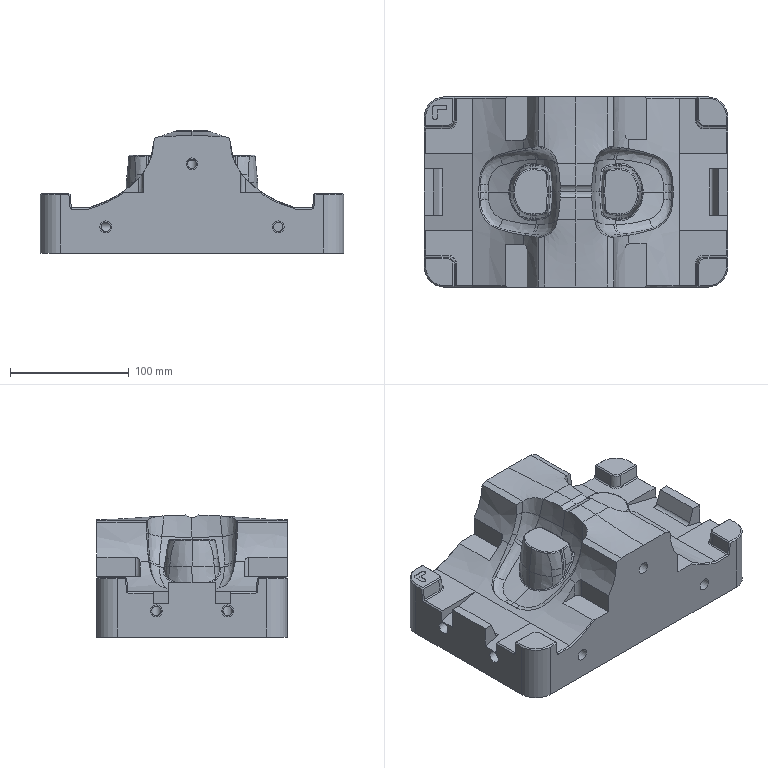NC program | NX | posted with a generic post | part box 255 x 160 x 102.619 mm
Lines 15545 to 16433 of 55104:
(CAVITY_MILL_COPY , TOOL : D10)
N31082 M6
N31084 G54
N31086 G17 G0 G90 X86.66 Y21.299 S1500 M3
N31088 G43 Z91.844 H0
N31090 Z85.846
N31092 G94 G1 Z85.646 F1800.
N31094 X89.16 Y21.298
N31096 X89.158 Y-0.058
N31098 X89.295
N31100 Y0.002
N31102 X89.297 Y41.955
N31104 G2 X94.006 Y47.232 R5.312
N31106 G3 X100.1 Y49.204 R16.171
N31108 X104.331 Y54.645 R8.734
N31110 X104.784 Y56.8 R26.441
N31112 G1 X105.098 Y58.674
N31114 G3 X104.51 Y104.627 R129.183
N31116 X102.821 Y108.479 R9.572
N31118 X100.066 Y110.819 R9.446
N31120 X93.854 Y112.789 R16.103
N31122 G2 X89.298 Y117.841 R5.31
N31124 G1 X89.294 Y118.621
N31126 X89.296 Y160.001
N31128 Y160.061
N31130 X89.158
N31132 Y159.958
N31134 X89.161 Y117.976
N31136 G3 X89.2 Y117.352 R5.
N31138 X90.013 Y115.113 R5.383
N31140 G2 X90.145 Y114.902 R9.958
N31142 G3 X90.785 Y114.064 R5.
N31144 X93.629 Y112.558 R5.
N31146 G1 X95.094 Y112.323
N31148 G2 X99.002 Y111.104 R14.358
N31150 X104.422 Y104.082 R9.828
N31152 X104.424 Y55.918 R128.176
N31154 X98.915 Y48.852 R9.828
N31156 X95.082 Y47.678 R14.563
N31158 G1 X93.64 Y47.447
N31160 G3 X90.623 Y45.749 R5.
N31162 X90.13 Y45.077 R5.
N31164 G2 X90.012 Y44.89 R9.958
N31166 G3 X89.2 Y42.653 R5.373
N31168 X89.161 Y42.03 R5.
N31170 G1 X89.16 Y21.298
N31172 X86.66 Y21.299
N31174 Z85.846
N31176 G0 Z102.92
N31178 X86.555
N31180 Z85.347
N31182 G1 Z85.147
N31184 X89.201 Y21.298
N31186 X89.2 Y41.382
N31188 X89.202 Y42.162
N31190 G2 X93.854 Y47.255 R5.308
N31192 G3 X100.1 Y49.283 R15.99
N31194 X104.244 Y54.645 R8.542
N31196 X104.784 Y57.295 R33.417
N31198 G1 X104.863 Y57.766
N31200 X104.988 Y58.546
N31202 X105.11 Y59.326
N31204 X105.252 Y60.106
N31206 G3 X104.724 Y103.017 R130.071
N31208 G1 X104.581 Y103.798
N31210 X104.433 Y104.578
N31212 G3 X102.442 Y108.83 R9.103
N31214 X99.934 Y110.819 R9.843
N31216 G1 X99.684 Y110.952
N31218 G3 X93.899 Y112.745 R16.307
N31220 G2 X89.203 Y117.841 R5.301
N31222 G1 X89.2 Y118.621
N31224 X89.202 Y159.941
N31226 Y160.001
N31228 Y160.061
N31230 X89.054
N31232 Y159.942
N31234 X89.056 Y117.968
N31236 G3 X89.094 Y117.358 R5.
N31238 X89.732 Y115.399 R5.375
N31240 G2 X89.909 Y115.067 R9.958
N31242 G3 X90.082 Y114.754 R5.
N31244 X93.586 Y112.375 R5.
N31246 G1 X95.064 Y112.138
N31248 G2 X98.921 Y110.935 R14.17
N31250 X104.238 Y104.047 R9.641
N31252 X104.24 Y55.953 R127.988
N31254 X98.836 Y49.022 R9.641
N31256 X95.052 Y47.863 R14.376
N31258 G1 X93.587 Y47.628
N31260 G3 X89.918 Y44.95 R5.
N31262 G2 X89.729 Y44.593 R9.958
N31264 G3 X89.097 Y42.678 R5.319
N31266 X89.056 Y42.041 R5.
N31268 G1 X89.053 Y0.039
N31270 Y-0.058
N31272 X89.202
N31274 Y0.002
N31276 X89.201 Y21.298
N31278 X86.555
N31280 Z85.347
N31282 G0 Z85.946
N31284 X86.45 Y21.299
N31286 Z84.848
N31288 G1 Z84.648
N31290 X89.091 Y21.298
N31292 Y41.382
N31294 X89.094 Y42.162
N31296 G2 X93.854 Y47.297 R5.324
N31298 G3 X100.1 Y49.362 R15.824
N31300 G1 X100.668 Y49.733
N31302 G3 X104.2 Y54.835 R8.209
N31304 X104.632 Y56.986 R55.03
N31306 X104.341 Y104.578 R129.924
N31308 X102.442 Y108.711 R8.905
N31310 X99.802 Y110.819 R9.712
N31312 G1 X99.319 Y111.07
N31314 G3 X93.854 Y112.714 R16.126
N31316 G2 X89.094 Y117.841 R5.304
N31318 G1 X89.092 Y118.621
N31320 X89.094 Y160.
N31322 Y160.061
N31324 X88.949
N31326 Y159.94
N31328 X88.952 Y117.933
N31330 G3 X88.986 Y117.353 R5.
N31332 X89.509 Y115.6 R5.296
N31334 G2 X89.671 Y115.26 R9.958
N31336 G3 X89.776 Y115.043 R5.
N31338 G1 X89.864 Y114.867
N31340 G3 X93.565 Y112.123 R5.
N31342 G1 X95.024 Y111.889
N31344 G2 X98.813 Y110.707 R13.918
N31346 X103.989 Y103.999 R9.388
N31348 X103.992 Y56. R127.736
N31350 X98.73 Y49.251 R9.388
N31352 X95.012 Y48.113 R14.123
N31354 G1 X93.568 Y47.881
N31356 G3 X89.867 Y45.137 R5.
N31358 G2 X89.761 Y44.928 R9.828
N31360 G3 X89.655 Y44.71 R5.
N31362 G2 X89.511 Y44.408 R9.958
N31364 G3 X88.984 Y42.631 R5.331
N31366 X88.951 Y42.065 R5.
N31368 G1 X88.949 Y0.039
N31370 Y-0.058
N31372 X89.094
N31374 Y0.002
N31376 X89.091 Y21.298
N31378 X86.45
N31380 Z84.848
N31382 G0 Z85.447
N31384 X86.336
N31386 Z84.348
N31388 G1 Z84.148
N31390 X88.977
N31392 Y42.162
N31394 G2 X93.854 Y47.339 R5.352
N31396 G3 X100.1 Y49.442 R15.667
N31398 G1 X100.617 Y49.781
N31400 G3 X104.131 Y54.928 R8.169
N31402 X104.814 Y58.546 R87.085
N31404 X105.876 Y93.655 R130.452
N31406 X104.244 Y104.578 R128.378
N31408 G1 X104.125 Y105.106
N31410 G3 X100.339 Y110.415 R8.397
N31412 X93.854 Y112.677 R15.953
N31414 G2 X88.978 Y117.841 R5.323
N31416 G1 Y160.001
N31418 Y160.061
N31420 X88.846
N31422 G2 X88.844 Y159.826 R9.958
N31424 G1 X88.837 Y159.348
N31426 Y117.925
N31428 G3 X88.863 Y117.415 R5.
N31430 X89.318 Y115.737 R5.369
N31432 G2 X89.438 Y115.463 R9.958
N31434 G1 X89.514 Y115.291
N31436 G2 X89.708 Y114.846 R9.828
N31438 G3 X93.547 Y111.791 R5.
N31440 G1 X94.972 Y111.562
N31442 G2 X98.67 Y110.409 R13.587
N31444 X103.665 Y103.937 R9.058
N31446 X103.667 Y56.062 R127.406
N31448 X98.591 Y49.551 R9.058
N31450 X94.96 Y48.439 R13.793
N31452 G1 X93.547 Y48.212
N31454 G3 X89.707 Y45.157 R5.
N31456 G2 X89.519 Y44.724 R9.828
N31458 G1 X89.443 Y44.553
N31460 G2 X89.314 Y44.258 R9.958
N31462 G3 X88.864 Y42.596 R5.269
N31464 X88.839 Y42.099 R5.
N31466 G1 X88.835 Y38.235
N31468 X88.837 Y0.042
N31470 Y-0.058
N31472 X88.978
N31474 Y0.002
N31476 X88.977 Y21.298
N31478 X86.336 Y21.299
N31480 Z84.348
N31482 G0 Z84.948
N31484 X86.213 Y21.298
N31486 Z83.849
N31488 G1 Z83.649
N31490 X88.861
N31492 Y42.054
N31494 G2 X93.308 Y47.287 R5.302
N31496 G1 X95.365 Y47.623
N31498 G3 X100.1 Y49.521 R16.573
N31500 X104.004 Y54.751 R8.29
N31502 G1 X104.148 Y55.425
N31504 G3 X104.146 Y104.578 R129.799
N31506 G1 X104.004 Y105.242
N31508 G3 X100.1 Y110.48 R8.259
N31510 X93.602 Y112.668 R16.117
N31512 G2 X88.861 Y117.964 R5.328
N31514 G1 X88.862 Y160.001
N31516 Y160.061
N31518 X88.716
N31520 G2 X88.714 Y159.745 R9.829
N31522 G1 X88.707 Y129.736
N31524 Y117.946
N31526 G3 X88.732 Y117.446 R5.
N31528 X89.142 Y115.84 R5.542
N31530 G2 X89.237 Y115.608 R9.958
N31532 G1 X89.292 Y115.474
N31534 G2 X89.581 Y114.715 R9.828
N31536 G3 X93.531 Y111.359 R5.
N31538 G1 X94.904 Y111.139
N31540 G2 X98.485 Y110.022 R13.158
N31542 X103.243 Y103.856 R8.628
N31544 X103.246 Y56.143 R126.976
N31546 X98.41 Y49.94 R8.628
N31548 X94.892 Y48.863 R13.364
N31550 G1 X93.532 Y48.644
N31552 G3 X89.581 Y45.289 R5.
N31554 G2 X89.291 Y44.526 R9.828
N31556 G1 X89.236 Y44.391
N31558 G2 X89.136 Y44.149 R9.958
N31560 G3 X88.736 Y42.563 R5.303
N31562 X88.715 Y42.106 R5.
N31564 G1 X88.712 Y38.236
N31566 X88.714 Y0.565
N31568 X88.721 Y0.166
N31570 G2 X88.722 Y-0.058 R9.958
N31572 G1 X88.862
N31574 Y0.002
N31576 X88.861 Y21.298
N31578 X86.213
N31580 Z83.849
N31582 G0 Z84.448
N31584 X86.083
N31586 Z83.35
N31588 G1 Z83.15
N31590 X88.739
N31592 Y42.162
N31594 G2 X93.073 Y47.295 R5.282
N31596 G1 X94.635 Y47.539
N31598 G3 X100.633 Y49.964 R15.487
N31600 X104.004 Y55.189 R8.207
N31602 X104.004 Y104.788 R130.22
N31604 X100.1 Y110.393 R8.228
N31606 X93.073 Y112.705 R16.762
N31608 G2 X88.739 Y117.841 R5.293
N31610 G1 X88.74 Y160.001
N31612 Y160.061
N31614 X88.599
N31616 G2 X88.598 Y159.851 R9.958
N31618 G1 X88.591 Y159.362
N31620 G3 X88.583 Y154.875 R10621.411
N31622 G1 X88.577 Y127.677
N31624 G3 X88.589 Y119.086 R10621.412
N31626 G1 X88.588 Y118.937
N31628 X88.577 Y118.043
N31630 G3 X88.585 Y117.664 R5.522
N31632 G1 X88.596 Y117.506
N31634 G3 X88.837 Y116.294 R5.672
N31636 G1 X88.887 Y116.144
N31638 G3 X88.994 Y115.861 R5.522
N31640 G1 X89.037 Y115.756
N31642 G2 X89.479 Y114.451 R9.828
N31644 G3 X93.523 Y110.783 R5.
N31646 G1 X94.813 Y110.575
N31648 G2 X98.24 Y109.507 R12.588
N31650 X102.683 Y103.749 R8.058
N31652 X102.686 Y56.25 R126.406
N31654 X98.169 Y50.457 R8.058
N31656 X94.801 Y49.426 R12.793
N31658 G1 X93.523 Y49.221
N31660 G3 X89.479 Y45.552 R5.
N31662 G2 X89.048 Y44.275 R9.828
N31664 G1 X89.006 Y44.168
N31666 X88.961 Y44.055
N31668 G3 X88.773 Y43.495 R5.
N31670 X88.671 Y43.044 R5.433
N31672 X88.591 Y42.161 R5.
N31674 X88.582 Y37.035 R10692.04
N31676 G1 X88.584 Y4.525
N31678 G3 X88.592 Y0.122 R10692.04
N31680 G1 Y-0.058
N31682 X88.74
N31684 Y0.002
N31686 X88.739 Y21.298
N31688 X86.083
N31690 Z83.35
N31692 G0 Z83.949
N31694 X85.942
N31696 Z82.851
N31698 G1 Z82.651
N31700 X88.603
N31702 Y42.162
N31704 G2 X93.073 Y47.341 R5.295
N31706 G1 X94.217 Y47.517
N31708 G3 X100.436 Y49.921 R15.541
N31710 X103.818 Y54.904 R7.932
N31712 X104.223 Y56.986 R72.136
N31714 X104.082 Y103.798 R130.312
N31716 G1 X104.004 Y104.247
N31718 G3 X103.202 Y106.918 R10.751
N31720 X100.1 Y110.295 R8.066
N31722 X93.073 Y112.658 R16.448
N31724 G2 X88.604 Y117.841 R5.304
N31726 G1 X88.605 Y160.001
N31728 Y160.061
N31730 X88.469
N31732 G2 X88.468 Y159.853 R9.828
N31734 G1 X88.461 Y159.363
N31736 G3 X88.445 Y147.332 R10621.542
N31738 X88.444 Y131.126 R17061.704
N31740 X88.459 Y119.085 R10621.542
N31742 G1 Y118.939
N31744 X88.447 Y118.044
N31746 G3 X88.851 Y115.871 R5.651
N31748 G2 X89.366 Y114.134 R9.828
N31750 G1 X89.387 Y114.032
N31752 X89.418 Y113.888
N31754 G3 X93.524 Y109.952 R5.
N31756 G1 X94.683 Y109.766
N31758 G2 X97.886 Y108.767 R11.768
N31760 X101.878 Y103.595 R7.238
N31762 X101.88 Y56.404 R125.586
N31764 X97.823 Y51.201 R7.238
N31766 X94.671 Y50.236 R11.973
N31768 G1 X93.525 Y50.052
N31770 G3 X89.418 Y46.116 R5.
N31772 G1 X89.385 Y45.96
N31774 X89.363 Y45.856
N31776 G2 X88.835 Y44.09 R9.828
N31778 G3 X88.472 Y42.499 R5.128
N31780 X88.461 Y42.185 R5.
N31782 X88.444 Y29.929 R10692.172
N31784 X88.444 Y12.465 R16785.576
N31786 X88.462 Y-0.058 R10692.172
N31788 G1 X88.605
N31790 Y0.002
N31792 X88.603 Y21.298
N31794 X85.942
N31796 Z82.851
N31798 G0 Z83.45
N31800 X85.813
N31802 Z82.351
N31804 G1 Z82.151
N31806 X88.468
N31808 Y42.162
N31810 G2 X93.073 Y47.387 R5.292
N31812 G3 X96.196 Y48.012 R20.197
N31814 X100.194 Y49.862 R17.051
N31816 X103.702 Y54.883 R7.902
N31818 G1 X103.818 Y55.425
N31820 G3 X103.817 Y104.578 R130.261
N31822 G1 X103.702 Y105.119
N31824 G3 X100.282 Y110.08 R7.872
N31826 X93.073 Y112.612 R16.29
N31828 G2 X88.468 Y117.841 R5.301
N31830 G1 X88.47 Y160.001
N31832 Y160.061
N31834 X88.334
N31836 G2 X88.333 Y159.838 R9.828
N31838 G1 X88.325 Y159.354
N31840 G3 X88.324 Y119.078 R17061.835
N31842 G1 X88.323 Y118.963
N31844 X88.312 Y117.935
N31846 G3 X88.668 Y115.964 R5.323
N31848 G2 X89.197 Y114.019 R9.829
N31850 X89.362 Y112.52 R9.641
N31852 G3 X93.567 Y107.739 R5.
N31854 G1 X94.338 Y107.615
N31856 G2 X96.948 Y106.801 R9.59
N31858 X99.739 Y103.186 R5.06
N31860 X99.741 Y56.813 R123.408
N31862 X96.905 Y53.176 R5.06
N31864 X94.326 Y52.386 R9.795
N31866 G1 X93.566 Y52.264
N31868 G3 X89.36 Y47.48 R5.
N31870 G2 X89.182 Y45.899 R9.642
N31872 X88.662 Y44.023 R9.828
N31874 G3 X88.325 Y42.225 R5.
N31876 X88.313 Y26.839 R16785.705
N31878 G1 Y16.041
N31880 G3 X88.326 Y-0.058 R16785.705
N31882 G1 X88.47
N31884 Y0.002
N31886 X88.468 Y21.298
N31888 X85.813
N31890 Z82.351
N31892 G0 Z82.951
N31894 X86.004 Y109.386
N31896 Z81.852
N31898 G1 Z81.652
N31900 X88.304 Y108.405
N31902 X99.055 Y104.624
N31904 G3 X97.698 Y106.293 R3.271
N31906 X92.972 Y108.047 R11.894
N31908 G2 X92.445 Y106.644 R13.888
N31910 X92.017 Y105.734 R13.558
N31912 X99.055 Y104.624 R31.845
N31914 G1 X98.683 Y103.274
N31916 X98.802 Y103.241
N31918 G2 X102.797 Y98.145 R5.47
N31920 G1 Y61.846
N31922 G2 X98.811 Y56.726 R5.281
N31924 X88.636 Y55.626 R36.633
N31926 X75.272 Y62.458 R17.612
N31928 X75.28 Y97.556 R28.687
N31930 X90.731 Y104.365 R17.827
N31932 X98.683 Y103.274 R30.445
N31934 G1 X99.055 Y104.624
N31936 X103.286 Y106.158
N31938 G3 X100.1 Y110.098 R7.771
N31940 X93.073 Y112.569 R16.394
N31942 G2 X88.323 Y117.841 R5.308
N31944 G1 X88.325 Y160.001
N31946 Y160.033
N31948 Y160.061
N31950 X88.192
N31952 G2 X88.19 Y159.842 R9.828
N31954 G1 X88.183 Y159.359
N31956 X88.177 Y117.798
N31958 G3 X88.183 Y117.556 R5.
N31960 X88.501 Y115.995 R5.235
N31962 G2 X89.002 Y114.045 R9.829
N31964 X89.047 Y111.1 R9.641
N31966 X88.68 Y109.399 R9.388
N31968 X88.304 Y108.405 R9.388
N31970 X88.019 Y107.8 R9.058
N31972 X87.523 Y106.955 R9.058
N31974 X86.317 Y105.466 R8.629
N31976 X84.429 Y104.055 R8.058
N31978 X83.259 Y103.518 R8.629
N31980 G1 X83.153 Y103.477
N31982 G3 X76.062 Y98.701 R18.435
N31984 X74.882 Y97.267 R18.113
N31986 X74.157 Y96.256 R28.762
N31988 X74.164 Y63.737 R28.838
N31990 X74.907 Y62.703 R28.762
N31992 X76.083 Y61.279 R18.17
N31994 X83.072 Y56.557 R18.432
N31996 G1 X83.206 Y56.508
N31998 G2 X85.129 Y55.521 R8.628
N32000 X85.749 Y55.054 R8.058
N32002 X87.63 Y52.883 R8.629
N32004 X88.019 Y52.204 R9.058
N32006 G1 X92.017 Y54.27
N32008 G2 X92.605 Y52.967 R13.558
N32010 X92.968 Y51.955 R13.888
N32012 G3 X97.694 Y53.704 R11.978
N32014 X99.038 Y55.34 R3.336
N32016 G2 X92.017 Y54.27 R38.033
N32018 G1 X88.019 Y52.204
N32020 G2 X88.433 Y51.281 R9.058
N32022 X88.677 Y50.601 R9.388
N32024 X89.045 Y48.9 R9.388
N32026 X88.995 Y45.919 R9.641
N32028 X88.496 Y43.993 R9.828
N32030 G3 X88.184 Y42.254 R5.
N32032 G1 Y0.563
N32034 X88.191 Y0.163
N32036 G2 X88.192 Y-0.058 R9.828
N32038 G1 X88.325
N32040 Y0.002
N32042 X88.322 Y41.382
N32044 X88.328 Y42.162
N32046 G2 X93.073 Y47.433 R5.294
N32048 G3 X100.1 Y49.901 R16.478
N32050 X103.528 Y54.645 R7.836
N32052 G1 X103.697 Y55.425
N32054 G3 X103.696 Y104.578 R130.035
N32056 G1 X103.528 Y105.358
N32058 G3 X103.286 Y106.158 R7.771
N32060 G1 X98.585 Y104.453
N32062 Z81.852
N32064 G0 Z82.451
N32066 X86.118 Y110.528
N32068 Z81.353
N32070 G1 Z81.153
N32072 X88.521 Y109.837
N32074 X88.525 Y109.853
N32076 X88.521 Y109.837
N32078 G2 X84.53 Y104.503 R9.388
N32080 X83.766 Y104.056 R9.641
N32082 X82.751 Y103.579 R9.828
N32084 G3 X80.813 Y102.667 R18.523
N32086 X75.314 Y98.093 R18.721
N32088 G1 X75.242 Y98.003
N32090 G3 X69.09 Y81.988 R29.512
N32092 X74.371 Y63.168 R29.436
N32094 X74.832 Y62.531 R29.46
N32096 X82.689 Y56.44 R18.687
N32098 G1 X82.842 Y56.377
N32100 G2 X83.253 Y56.196 R9.828
N32102 X84.763 Y55.342 R9.641
N32104 X88.483 Y50.286 R9.388
N32106 X88.911 Y46.938 R9.641
N32108 X88.334 Y43.957 R9.828
N32110 G3 X88.037 Y42.261 R5.
N32112 G1 X88.035 Y0.659
N32114 X88.036 Y0.567
N32116 X88.043 Y0.182
N32118 G2 X88.044 Y-0.058 R9.828
N32120 G1 X88.165
N32122 Y0.002
N32124 X88.163 Y41.382
N32126 X88.179 Y42.162
N32128 G2 X92.292 Y47.338 R5.247
N32130 G1 X93.854 Y47.591
N32132 G3 X99.319 Y49.519 R16.879
N32134 X101.657 Y51.344 R9.657
N32136 X103.398 Y54.648 R7.033
N32138 X103.943 Y57.464 R57.449
N32140 G2 X101.918 Y56.668 R13.324
N32142 X93.664 Y55.337 R31.617
N32144 G1 X90.731 Y55.257
N32146 X89.95
N32148 X89.169 Y55.266
N32150 G2 X75.698 Y61.667 R18.154
N32152 X75.698 Y98.336 R29.03
N32154 X89.169 Y104.739 R18.166
N32156 G1 X89.95 Y104.746
N32158 X90.731 Y104.747
N32160 X93.679 Y104.666
N32162 G2 X102.894 Y103.017 R31.4
N32164 G1 X103.944 Y102.537
N32166 G3 X103.397 Y105.358 R49.05
N32168 X100.1 Y109.992 R7.647
N32170 X93.073 Y112.523 R16.334
N32172 G2 X88.163 Y117.841 R5.344
N32174 G1 X88.166 Y160.001
N32176 Y160.061
N32178 X88.044
N32180 G2 X88.042 Y159.818 R9.828
N32182 G1 X88.035 Y159.435
N32184 X88.034 Y159.343
N32186 X88.035 Y117.751
N32188 X88.036 Y117.624
N32190 G3 X88.336 Y116.023 R5.119
N32192 G2 X88.904 Y113.18 R9.828
N32194 X88.525 Y109.853 R9.641
N32196 G1 X86.125 Y110.551
N32198 Z81.353
N32200 G0 Z81.952
N32202 X85.924 Y110.637
N32204 Z80.854
N32206 G1 Z80.654
N32208 X88.318 Y109.916
N32210 G2 X86.124 Y106.109 R9.641
N32212 X83.435 Y104.053 R9.828
N32214 X82.557 Y103.634 R9.958
N32216 G3 X75.547 Y98.503 R18.642
N32218 X75.178 Y98.049 R18.565
N32220 X73.511 Y95.686 R29.294
N32222 X69.695 Y86.535 R29.62
N32224 X69.31 Y75.461 R29.294
N32226 X75.221 Y61.895 R29.536
N32228 X82.555 Y56.369 R18.622
N32230 G2 X83.318 Y56.011 R9.958
N32232 X86.846 Y53.017 R9.828
N32234 X88.729 Y47.362 R9.641
N32236 X88.165 Y43.946 R9.828
N32238 G3 X87.878 Y42.276 R5.
N32240 G1 X87.871 Y0.564
N32242 X87.878 Y0.175
N32244 G2 X87.879 Y-0.058 R9.828
N32246 G1 X88.006
N32248 Y0.002
N32250 X88.004 Y41.382
N32252 X88.055 Y42.942
N32254 G2 X91.62 Y47.233 R5.361
N32256 X93.073 Y47.525 R10.819
N32258 G1 X93.78 Y47.623
N32260 G3 X100.071 Y50.099 R16.547
N32262 X103.325 Y54.944 R7.517
N32264 G1 X103.733 Y57.032
N32266 G2 X102.442 Y56.558 R8.207
N32268 X93.073 Y55.136 R33.899
N32270 G1 X90.84 Y55.111
N32272 G2 X89.284 Y55.117 R81.867
N32274 X74.98 Y62.447 R18.151
N32276 X75.59 Y98.336 R29.136
N32278 X89.284 Y104.89 R18.183
N32280 X90.839 Y104.895 R83.005
N32282 G1 X93.073 Y104.868
N32284 G2 X102.499 Y103.426 R33.793
N32286 X103.735 Y102.963 R10.158
N32288 G1 X103.325 Y105.061
N32290 G3 X100.169 Y109.826 R7.479
N32292 X93.073 Y112.477 R16.177
N32294 G1 X92.564 Y112.552
N32296 G2 X88.004 Y117.831 R5.335
N32298 G1 X88.006 Y160.001
N32300 Y160.061
N32302 X87.879
N32304 G2 X87.877 Y159.827 R9.828
N32306 G1 X87.869 Y159.348
N32308 X87.87 Y117.788
N32310 X87.873 Y117.604
N32312 G3 X88.171 Y116.037 R5.303
N32314 G2 X88.728 Y112.637 R9.828
N32316 X88.318 Y109.916 R9.641
N32318 G1 X85.924 Y110.637
N32320 Z80.854
N32322 G0 Z81.453
N32324 X85.734 Y110.7
N32326 Z80.354
N32328 G1 Z80.154
N32330 X88.126 Y109.974
N32332 G2 X87.208 Y107.881 R9.641
N32334 X83.005 Y103.978 R9.828
N32336 X82.431 Y103.711 R9.958
N32338 G3 X75.57 Y98.649 R18.642
N32340 G1 X75.511 Y98.578
N32342 G3 X71.135 Y91.284 R29.337
N32344 X72.127 Y66.574 R29.37
N32346 X74.338 Y62.95 R29.337
N32348 G1 X74.882 Y62.205
N32350 G3 X75.362 Y61.591 R18.711
N32352 X82.438 Y56.293 R18.74
N32354 G2 X83.307 Y55.87 R9.958
N32356 X86.924 Y52.578 R9.828
N32358 X88.478 Y46.114 R9.641
N32360 X87.993 Y43.962 R9.828
N32362 G3 X87.717 Y42.28 R5.
N32364 G1 X87.706 Y0.562
N32366 X87.712 Y0.167
N32368 G2 X87.714 Y-0.058 R9.828
N32370 G1 X87.846
N32372 Y0.002
N32374 X87.845 Y41.382
N32376 X87.857 Y42.162
N32378 G2 X92.292 Y47.45 R5.259
N32380 G3 X94.818 Y47.91 R24.573
N32382 X100.114 Y50.257 R15.744
N32384 X103.223 Y55.071 R7.446
N32386 G1 X103.5 Y56.601
N32388 X103.544 Y56.797
N32390 G2 X96.196 Y55.187 R30.128
N32392 X90.844 Y54.981 R49.122
N32394 X89.292 Y54.986 R81.997
N32396 X75.896 Y61.183 R18.218
N32398 X75.896 Y98.82 R29.187
N32400 X89.292 Y105.02 R18.234
N32402 X90.843 Y105.025 R83.136
N32404 G1 X93.286 Y104.992
N32406 G2 X102.457 Y103.578 R33.478
N32408 X103.542 Y103.198 R12.643
N32410 G1 X103.288 Y104.578
N32412 X103.179 Y105.115
N32414 G3 X100.082 Y109.766 R7.395
N32416 G1 X99.679 Y110.039
N32418 G3 X92.292 Y112.536 R16.969
N32420 G2 X87.844 Y117.841 R5.327
N32422 G1 X87.847 Y160.001
N32424 Y160.061
N32426 X87.713
N32428 G2 X87.712 Y159.834 R9.828
N32430 G1 X87.705 Y159.353
N32432 Y117.757
N32434 X87.706 Y117.65
N32436 G3 X87.995 Y116.04 R5.257
N32438 G2 X88.523 Y113.36 R9.828
N32440 X88.126 Y109.974 R9.641
N32442 G1 X85.734 Y110.7
N32444 Z80.354
N32446 G0 Z80.954
N32448 X85.546 Y110.753
N32450 Z79.855
N32452 G1 Z79.655
N32454 X87.939 Y110.03
N32456 G2 X86.379 Y106.977 R9.641
N32458 X83.21 Y104.232 R9.828
N32460 X82.312 Y103.783 R9.958
N32462 G3 X75.863 Y99.116 R18.774
N32464 G1 X75.772 Y99.011
N32466 G3 X72.458 Y94.203 R29.413
N32468 X74.257 Y62.939 R29.448
N32470 G1 X74.879 Y62.089
N32472 G3 X75.316 Y61.528 R18.666
N32474 X82.314 Y56.219 R18.788
N32476 G2 X83.055 Y55.857 R9.958
N32478 X87.01 Y52.086 R9.828
N32480 X88.322 Y46.459 R9.641
N32482 X87.817 Y43.96 R9.828
N32484 G3 X87.548 Y42.281 R5.
N32486 G1 X87.541 Y0.561
N32488 X87.547 Y0.16
N32490 G2 X87.548 Y-0.058 R9.828
N32492 G1 X87.686
N32494 Y0.002
N32496 Y0.006
N32498 Y0.062
N32500 X87.689 Y42.162
N32502 G2 X92.292 Y47.506 R5.274
N32504 G3 X98.538 Y49.404 R17.69
N32506 X100.881 Y51.022 R10.385
N32508 X102.96 Y54.645 R6.815
N32510 G1 X103.355 Y56.577
N32512 G2 X93.073 Y54.879 R33.526
N32514 G1 X90.847 Y54.853
N32516 G2 X89.3 Y54.858 R82.125
N32518 X75.896 Y61.061 R18.235
N32520 X75.896 Y98.943 R29.302
N32522 X89.3 Y105.147 R18.28
N32524 X90.846 Y105.152 R83.262
N32526 G1 X93.396 Y105.115
N32528 G2 X103.353 Y103.419 R32.929
N32530 G1 X102.974 Y105.358
N32532 G3 X100.1 Y109.633 R7.339
N32534 X92.292 Y112.483 R16.558
N32536 G2 X87.685 Y117.841 R5.313
N32538 G1 X87.687 Y159.978
N32540 Y160.001
N32542 Y160.061
N32544 X87.548
N32546 G2 X87.547 Y159.841 R9.828
N32548 G1 X87.54 Y159.358
N32550 Y117.72
N32552 G3 X87.822 Y116.004 R5.371
N32554 G2 X88.137 Y114.835 R9.828
N32556 X87.939 Y110.03 R9.641
N32558 G1 X85.546 Y110.753
N32560 Z79.855
N32562 G0 Z80.454
N32564 X85.348 Y110.809
N32566 Z79.356
N32568 G1 Z79.156
N32570 X87.742 Y110.09
N32572 G2 X86.817 Y107.972 R9.641
N32574 X83.202 Y104.376 R9.828
N32576 X82.178 Y103.845 R9.958
N32578 G3 X76.582 Y99.997 R18.835
N32580 X75.338 Y98.599 R18.422
N32582 G1 X74.917 Y98.075
N32584 X74.853 Y97.993
N32586 G3 X74.18 Y62.929 R29.503
N32588 G1 X74.892 Y61.95
N32590 G3 X75.393 Y61.312 R18.628
N32592 X82.176 Y56.159 R18.742
N32594 G2 X83.254 Y55.596 R9.958
N32596 X86.367 Y52.736 R9.828
N32598 X87.921 Y45.014 R9.641
N32600 X87.631 Y43.963 R9.828
N32602 G3 X87.37 Y42.283 R5.
N32604 G1 Y0.657
N32606 Y0.567
N32608 X87.377 Y0.179
N32610 G2 X87.379 Y-0.058 R9.828
N32612 G1 X87.512
N32614 Y0.002
N32616 X87.511 Y42.162
N32618 G2 X92.292 Y47.561 R5.301
N32620 G3 X99.319 Y49.952 R17.374
N32622 X100.69 Y51.004 R12.063
N32624 X102.804 Y54.65 R6.712
N32626 G1 X103.129 Y56.205
N32628 X103.16 Y56.371
N32630 G2 X93.073 Y54.754 R34.742
N32632 G1 X90.85 Y54.729
N32634 G2 X89.308 Y54.734 R82.248
N32636 X75.896 Y60.938 R18.299
N32638 X69.632 Y86.633 R29.425
N32640 X75.896 Y99.065 R29.777
N32642 X89.308 Y105.27 R18.312
N32644 X90.849 Y105.276 R83.386
N32646 G1 X93.269 Y105.241
N32648 G2 X103.161 Y103.632 R34.255
N32650 G1 X102.862 Y105.16
N32652 G3 X100.253 Y109.376 R7.02
N32654 X96.977 Y111.239 R13.64
N32656 X92.292 Y112.434 R17.565
N32658 G2 X87.984 Y115.501 R5.389
N32660 X87.51 Y117.841 R5.585
N32662 G1 X87.513 Y159.985
N32664 Y160.001
N32666 Y160.051
N32668 Y160.061
N32670 X87.379
N32672 G2 X87.377 Y159.821 R9.828
N32674 G1 X87.37 Y159.436
N32676 X87.369 Y159.343
N32678 X87.37 Y117.666
N32680 G3 X87.632 Y116.036 R5.028
N32682 G2 X88.087 Y113.96 R9.828
N32684 X87.742 Y110.09 R9.641
N32686 G1 X85.348 Y110.809
N32688 Z79.356
N32690 G0 Z79.955
N32692 X85.158 Y110.861
N32694 Z78.857
N32696 G1 Z78.657
N32698 X87.554 Y110.146
N32700 G2 X86.262 Y107.445 R9.641
N32702 X83.018 Y104.418 R9.828
N32704 X82.028 Y103.898 R9.958
N32706 G3 X75.524 Y98.946 R18.499
N32708 X75.323 Y98.7 R18.363
N32710 G1 X74.834 Y98.089
N32712 X74.767 Y98.004
N32714 G3 X74.105 Y62.916 R29.595
N32716 G1 X74.967 Y61.728
N32718 G3 X75.526 Y61.034 R18.828
N32720 X82.034 Y56.109 R18.705
N32722 G2 X83.375 Y55.368 R9.958
N32724 X86.331 Y52.457 R9.828
N32726 X87.513 Y44.205 R9.641
N32728 X87.448 Y44. R9.828
N32730 G3 X87.251 Y43.2 R5.421
N32732 X87.186 Y42.557 R5.
N32734 X87.182 Y42.283 R5.177
N32736 G1 Y0.656
N32738 X87.183 Y0.565
N32740 X87.19 Y0.176
N32742 G2 X87.191 Y-0.058 R9.641
N32744 G1 X87.323
N32746 Y0.002
N32748 X87.321 Y42.31
N32750 G2 X91.285 Y47.43 R5.288
N32752 X92.292 Y47.617 R7.411
N32754 G3 X98.538 Y49.616 R17.398
N32756 X101.045 Y51.524 R10.002
N32758 X102.645 Y54.645 R6.728
N32760 G1 X102.959 Y56.175
N32762 G2 X93.124 Y54.637 R35.033
N32764 G1 X90.853 Y54.609
N32766 G2 X89.95 Y54.608 R82.369
N32768 G1 X89.371 Y54.613
N32770 G2 X75.842 Y60.887 R18.291
N32772 X68.817 Y81.172 R29.707
N32774 X75.896 Y99.178 R29.803
N32776 X89.315 Y105.391 R18.295
N32778 X90.852 Y105.396 R83.506
N32780 G1 X93.137 Y105.366
N32782 G2 X102.958 Y103.829 R35.05
N32784 G1 X102.654 Y105.358
N32786 G3 X100.044 Y109.393 R6.911
N32788 X97.104 Y111.089 R14.377
N32790 X92.128 Y112.404 R17.633
N32792 G2 X88.87 Y113.94 R5.582
N32794 X87.321 Y117.841 R5.4
N32796 G1 X87.323 Y160.001
N32798 Y160.061
N32800 X87.191
N32802 G2 X87.19 Y159.824 R9.641
N32804 G1 X87.183 Y159.437
N32806 X87.182 Y159.345
N32808 Y117.667
N32810 X87.184 Y117.519
N32812 G3 X87.23 Y116.94 R5.
N32814 X87.463 Y115.948 R5.569
N32816 G2 X87.554 Y110.146 R9.641
N32818 G1 X85.158 Y110.861
N32820 Z78.857
N32822 G0 Z79.456
N32824 X84.958 Y110.912
N32826 Z78.358
N32828 G1 Z78.158
N32830 X87.356 Y110.204
N32832 G2 X85.908 Y107.265 R9.641
N32834 X83.289 Y104.741 R9.828
N32836 X81.885 Y103.944 R9.958
N32838 G3 X75.263 Y98.748 R18.44
N32840 G1 X74.893 Y98.286
N32842 X74.772 Y98.128
N32844 X74.657 Y97.971
N32846 X73.991 Y97.046
N32848 G3 X74.025 Y62.911 R29.607
N32850 G1 X74.661 Y62.03
N32852 G3 X76.135 Y60.234 R18.808